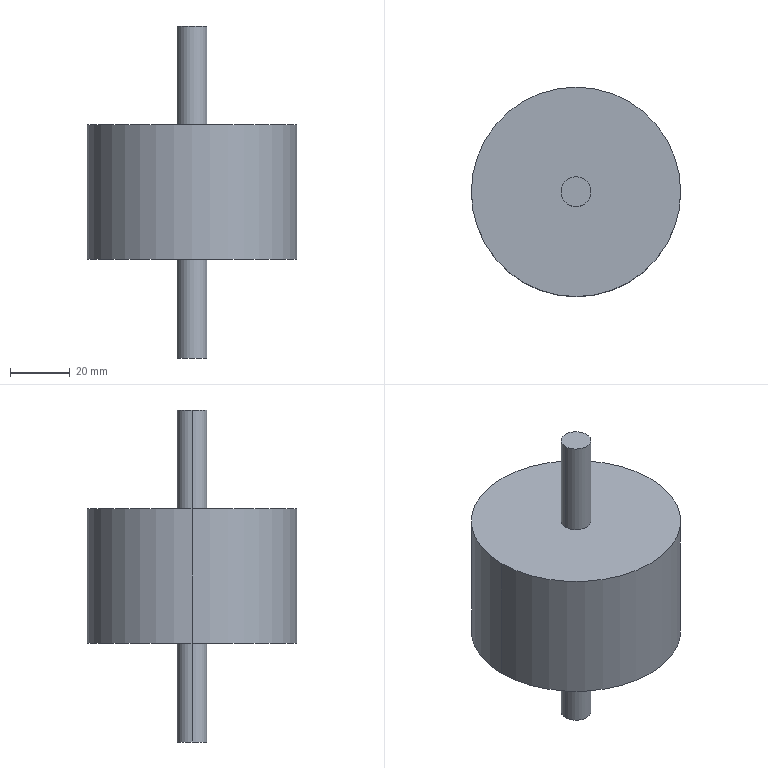Part | 1 solid | 10 faces | box 70 x 70 x 111 mm | volume 178364 mm3 | cylinder 6 | plane 4 | commonest cylinder face diameters 10 x4 70 x2
STEP:
#1=CARTESIAN_POINT('',(-5.,0.,-33.));
#2=VERTEX_POINT('',#1);
#3=CARTESIAN_POINT('',(5.,0.,-33.));
#4=VERTEX_POINT('',#3);
#5=CARTESIAN_POINT('',(0.,0.,-33.));
#6=DIRECTION('',(0.,0.,-1.));
#7=DIRECTION('',(-1.,0.,0.));
#8=AXIS2_PLACEMENT_3D('',#5,#6,#7);
#9=CIRCLE('',#8,5.);
#10=EDGE_CURVE('',#2,#4,#9,.T.);
#11=ORIENTED_EDGE('',*,*,#10,.F.);
#12=CARTESIAN_POINT('',(-5.,0.,0.));
#13=VERTEX_POINT('',#12);
#14=CARTESIAN_POINT('',(-5.,0.,-33.));
#15=DIRECTION('',(0.,0.,1.));
#16=VECTOR('',#15,1000.);
#17=LINE('',#14,#16);
#18=EDGE_CURVE('',#2,#13,#17,.T.);
#19=ORIENTED_EDGE('',*,*,#18,.T.);
#20=CARTESIAN_POINT('',(5.,0.,0.));
#21=VERTEX_POINT('',#20);
#22=CARTESIAN_POINT('',(0.,0.,0.));
#23=DIRECTION('',(0.,0.,-1.));
#24=DIRECTION('',(1.,0.,0.));
#25=AXIS2_PLACEMENT_3D('',#22,#23,#24);
#26=CIRCLE('',#25,5.);
#27=EDGE_CURVE('',#13,#21,#26,.T.);
#28=ORIENTED_EDGE('',*,*,#27,.T.);
#29=CARTESIAN_POINT('',(5.,0.,-33.));
#30=DIRECTION('',(0.,0.,1.));
#31=VECTOR('',#30,1000.);
#32=LINE('',#29,#31);
#33=EDGE_CURVE('',#4,#21,#32,.T.);
#34=ORIENTED_EDGE('',*,*,#33,.F.);
#35=EDGE_LOOP('',(#11,#19,#28,#34));
#36=FACE_OUTER_BOUND('',#35,.T.);
#37=CARTESIAN_POINT('',(0.,0.,-33.));
#38=DIRECTION('',(0.,0.,1.));
#39=DIRECTION('',(1.,0.,0.));
#40=AXIS2_PLACEMENT_3D('',#37,#38,#39);
#41=CYLINDRICAL_SURFACE('',#40,5.);
#42=ADVANCED_FACE('',(#36),#41,.T.);
#43=CARTESIAN_POINT('',(5.,0.,78.));
#44=VERTEX_POINT('',#43);
#45=CARTESIAN_POINT('',(-5.,0.,78.));
#46=VERTEX_POINT('',#45);
#47=CARTESIAN_POINT('',(0.,0.,78.));
#48=DIRECTION('',(0.,0.,1.));
#49=DIRECTION('',(1.,0.,0.));
#50=AXIS2_PLACEMENT_3D('',#47,#48,#49);
#51=CIRCLE('',#50,5.);
#52=EDGE_CURVE('',#44,#46,#51,.T.);
#53=ORIENTED_EDGE('',*,*,#52,.F.);
#54=CARTESIAN_POINT('',(5.,0.,45.));
#55=VERTEX_POINT('',#54);
#56=CARTESIAN_POINT('',(5.,0.,78.));
#57=DIRECTION('',(0.,0.,-1.));
#58=VECTOR('',#57,1000.);
#59=LINE('',#56,#58);
#60=EDGE_CURVE('',#44,#55,#59,.T.);
#61=ORIENTED_EDGE('',*,*,#60,.T.);
#62=CARTESIAN_POINT('',(-5.,0.,45.));
#63=VERTEX_POINT('',#62);
#64=CARTESIAN_POINT('',(0.,0.,45.));
#65=DIRECTION('',(0.,0.,1.));
#66=DIRECTION('',(1.,0.,0.));
#67=AXIS2_PLACEMENT_3D('',#64,#65,#66);
#68=CIRCLE('',#67,5.);
#69=EDGE_CURVE('',#55,#63,#68,.T.);
#70=ORIENTED_EDGE('',*,*,#69,.T.);
#71=CARTESIAN_POINT('',(-5.,0.,78.));
#72=DIRECTION('',(0.,0.,-1.));
#73=VECTOR('',#72,1000.);
#74=LINE('',#71,#73);
#75=EDGE_CURVE('',#46,#63,#74,.T.);
#76=ORIENTED_EDGE('',*,*,#75,.F.);
#77=EDGE_LOOP('',(#53,#61,#70,#76));
#78=FACE_OUTER_BOUND('',#77,.T.);
#79=CARTESIAN_POINT('',(0.,0.,78.));
#80=DIRECTION('',(0.,0.,-1.));
#81=DIRECTION('',(-1.,0.,0.));
#82=AXIS2_PLACEMENT_3D('',#79,#80,#81);
#83=CYLINDRICAL_SURFACE('',#82,5.);
#84=ADVANCED_FACE('',(#78),#83,.T.);
#85=CARTESIAN_POINT('',(35.,0.,45.));
#86=VERTEX_POINT('',#85);
#87=CARTESIAN_POINT('',(-35.,0.,45.));
#88=VERTEX_POINT('',#87);
#89=CARTESIAN_POINT('',(0.,0.,45.));
#90=DIRECTION('',(0.,0.,1.));
#91=DIRECTION('',(1.,0.,0.));
#92=AXIS2_PLACEMENT_3D('',#89,#90,#91);
#93=CIRCLE('',#92,35.);
#94=EDGE_CURVE('',#86,#88,#93,.T.);
#95=ORIENTED_EDGE('',*,*,#94,.F.);
#96=CARTESIAN_POINT('',(35.,0.,0.));
#97=VERTEX_POINT('',#96);
#98=CARTESIAN_POINT('',(35.,0.,45.));
#99=DIRECTION('',(0.,0.,-1.));
#100=VECTOR('',#99,1000.);
#101=LINE('',#98,#100);
#102=EDGE_CURVE('',#86,#97,#101,.T.);
#103=ORIENTED_EDGE('',*,*,#102,.T.);
#104=CARTESIAN_POINT('',(-35.,0.,0.));
#105=VERTEX_POINT('',#104);
#106=CARTESIAN_POINT('',(0.,0.,0.));
#107=DIRECTION('',(0.,0.,1.));
#108=DIRECTION('',(1.,0.,0.));
#109=AXIS2_PLACEMENT_3D('',#106,#107,#108);
#110=CIRCLE('',#109,35.);
#111=EDGE_CURVE('',#97,#105,#110,.T.);
#112=ORIENTED_EDGE('',*,*,#111,.T.);
#113=CARTESIAN_POINT('',(-35.,0.,45.));
#114=DIRECTION('',(0.,0.,-1.));
#115=VECTOR('',#114,1000.);
#116=LINE('',#113,#115);
#117=EDGE_CURVE('',#88,#105,#116,.T.);
#118=ORIENTED_EDGE('',*,*,#117,.F.);
#119=EDGE_LOOP('',(#95,#103,#112,#118));
#120=FACE_OUTER_BOUND('',#119,.T.);
#121=CARTESIAN_POINT('',(0.,0.,45.));
#122=DIRECTION('',(0.,0.,-1.));
#123=DIRECTION('',(-1.,0.,0.));
#124=AXIS2_PLACEMENT_3D('',#121,#122,#123);
#125=CYLINDRICAL_SURFACE('',#124,35.);
#126=ADVANCED_FACE('',(#120),#125,.T.);
#127=ORIENTED_EDGE('',*,*,#102,.F.);
#128=CARTESIAN_POINT('',(0.,0.,45.));
#129=DIRECTION('',(0.,0.,1.));
#130=DIRECTION('',(1.,0.,0.));
#131=AXIS2_PLACEMENT_3D('',#128,#129,#130);
#132=CIRCLE('',#131,35.);
#133=EDGE_CURVE('',#88,#86,#132,.T.);
#134=ORIENTED_EDGE('',*,*,#133,.F.);
#135=ORIENTED_EDGE('',*,*,#117,.T.);
#136=CARTESIAN_POINT('',(0.,0.,0.));
#137=DIRECTION('',(0.,0.,1.));
#138=DIRECTION('',(1.,0.,0.));
#139=AXIS2_PLACEMENT_3D('',#136,#137,#138);
#140=CIRCLE('',#139,35.);
#141=EDGE_CURVE('',#105,#97,#140,.T.);
#142=ORIENTED_EDGE('',*,*,#141,.T.);
#143=EDGE_LOOP('',(#127,#134,#135,#142));
#144=FACE_OUTER_BOUND('',#143,.T.);
#145=CARTESIAN_POINT('',(0.,0.,45.));
#146=DIRECTION('',(0.,0.,-1.));
#147=DIRECTION('',(-1.,0.,0.));
#148=AXIS2_PLACEMENT_3D('',#145,#146,#147);
#149=CYLINDRICAL_SURFACE('',#148,35.);
#150=ADVANCED_FACE('',(#144),#149,.T.);
#151=CARTESIAN_POINT('',(0.,0.,45.));
#152=DIRECTION('',(0.,0.,1.));
#153=DIRECTION('',(1.,0.,0.));
#154=AXIS2_PLACEMENT_3D('',#151,#152,#153);
#155=CIRCLE('',#154,5.);
#156=EDGE_CURVE('',#63,#55,#155,.T.);
#157=ORIENTED_EDGE('',*,*,#156,.F.);
#158=ORIENTED_EDGE('',*,*,#69,.F.);
#159=EDGE_LOOP('',(#157,#158));
#160=FACE_BOUND('',#159,.T.);
#161=ORIENTED_EDGE('',*,*,#133,.T.);
#162=ORIENTED_EDGE('',*,*,#94,.T.);
#163=EDGE_LOOP('',(#161,#162));
#164=FACE_OUTER_BOUND('',#163,.T.);
#165=CARTESIAN_POINT('',(0.,0.,45.));
#166=DIRECTION('',(0.,0.,1.));
#167=DIRECTION('',(1.,0.,0.));
#168=AXIS2_PLACEMENT_3D('',#165,#166,#167);
#169=PLANE('',#168);
#170=ADVANCED_FACE('',(#160,#164),#169,.T.);
#171=CARTESIAN_POINT('',(0.,0.,0.));
#172=DIRECTION('',(0.,0.,-1.));
#173=DIRECTION('',(1.,0.,0.));
#174=AXIS2_PLACEMENT_3D('',#171,#172,#173);
#175=CIRCLE('',#174,5.);
#176=EDGE_CURVE('',#21,#13,#175,.T.);
#177=ORIENTED_EDGE('',*,*,#176,.F.);
#178=ORIENTED_EDGE('',*,*,#27,.F.);
#179=EDGE_LOOP('',(#177,#178));
#180=FACE_BOUND('',#179,.T.);
#181=ORIENTED_EDGE('',*,*,#141,.F.);
#182=ORIENTED_EDGE('',*,*,#111,.F.);
#183=EDGE_LOOP('',(#181,#182));
#184=FACE_OUTER_BOUND('',#183,.T.);
#185=CARTESIAN_POINT('',(0.,0.,0.));
#186=DIRECTION('',(0.,0.,1.));
#187=DIRECTION('',(1.,0.,0.));
#188=AXIS2_PLACEMENT_3D('',#185,#186,#187);
#189=PLANE('',#188);
#190=ADVANCED_FACE('',(#180,#184),#189,.F.);
#191=ORIENTED_EDGE('',*,*,#60,.F.);
#192=CARTESIAN_POINT('',(0.,0.,78.));
#193=DIRECTION('',(0.,0.,1.));
#194=DIRECTION('',(1.,0.,0.));
#195=AXIS2_PLACEMENT_3D('',#192,#193,#194);
#196=CIRCLE('',#195,5.);
#197=EDGE_CURVE('',#46,#44,#196,.T.);
#198=ORIENTED_EDGE('',*,*,#197,.F.);
#199=ORIENTED_EDGE('',*,*,#75,.T.);
#200=ORIENTED_EDGE('',*,*,#156,.T.);
#201=EDGE_LOOP('',(#191,#198,#199,#200));
#202=FACE_OUTER_BOUND('',#201,.T.);
#203=CARTESIAN_POINT('',(0.,0.,78.));
#204=DIRECTION('',(0.,0.,-1.));
#205=DIRECTION('',(-1.,0.,0.));
#206=AXIS2_PLACEMENT_3D('',#203,#204,#205);
#207=CYLINDRICAL_SURFACE('',#206,5.);
#208=ADVANCED_FACE('',(#202),#207,.T.);
#209=ORIENTED_EDGE('',*,*,#197,.T.);
#210=ORIENTED_EDGE('',*,*,#52,.T.);
#211=EDGE_LOOP('',(#209,#210));
#212=FACE_OUTER_BOUND('',#211,.T.);
#213=CARTESIAN_POINT('',(0.,0.,78.));
#214=DIRECTION('',(0.,0.,1.));
#215=DIRECTION('',(1.,0.,0.));
#216=AXIS2_PLACEMENT_3D('',#213,#214,#215);
#217=PLANE('',#216);
#218=ADVANCED_FACE('',(#212),#217,.T.);
#219=ORIENTED_EDGE('',*,*,#18,.F.);
#220=CARTESIAN_POINT('',(0.,0.,-33.));
#221=DIRECTION('',(0.,0.,-1.));
#222=DIRECTION('',(-1.,0.,0.));
#223=AXIS2_PLACEMENT_3D('',#220,#221,#222);
#224=CIRCLE('',#223,5.);
#225=EDGE_CURVE('',#4,#2,#224,.T.);
#226=ORIENTED_EDGE('',*,*,#225,.F.);
#227=ORIENTED_EDGE('',*,*,#33,.T.);
#228=ORIENTED_EDGE('',*,*,#176,.T.);
#229=EDGE_LOOP('',(#219,#226,#227,#228));
#230=FACE_OUTER_BOUND('',#229,.T.);
#231=CARTESIAN_POINT('',(0.,0.,-33.));
#232=DIRECTION('',(0.,0.,1.));
#233=DIRECTION('',(1.,0.,0.));
#234=AXIS2_PLACEMENT_3D('',#231,#232,#233);
#235=CYLINDRICAL_SURFACE('',#234,5.);
#236=ADVANCED_FACE('',(#230),#235,.T.);
#237=ORIENTED_EDGE('',*,*,#225,.T.);
#238=ORIENTED_EDGE('',*,*,#10,.T.);
#239=EDGE_LOOP('',(#237,#238));
#240=FACE_OUTER_BOUND('',#239,.T.);
#241=CARTESIAN_POINT('',(0.,0.,-33.));
#242=DIRECTION('',(0.,0.,-1.));
#243=DIRECTION('',(-1.,0.,0.));
#244=AXIS2_PLACEMENT_3D('',#241,#242,#243);
#245=PLANE('',#244);
#246=ADVANCED_FACE('',(#240),#245,.T.);
#247=CLOSED_SHELL('',(#42,#84,#126,#150,#170,#190,#208,#218,#236,#246));
#248=MANIFOLD_SOLID_BREP('',#247);
#249=CARTESIAN_POINT('',(0.,0.,0.));
#250=DIRECTION('',(0.,0.,1.));
#251=DIRECTION('',(1.,0.,0.));
#252=AXIS2_PLACEMENT_3D('',#249,#250,#251);
#253=(LENGTH_UNIT()NAMED_UNIT(*)SI_UNIT(.MILLI.,.METRE.));
#254=UNCERTAINTY_MEASURE_WITH_UNIT(LENGTH_MEASURE(0.00001),#253,'','');
#255=(NAMED_UNIT(*)PLANE_ANGLE_UNIT()SI_UNIT($,.RADIAN.));
#256=(NAMED_UNIT(*)SI_UNIT($,.STERADIAN.)SOLID_ANGLE_UNIT());
#257=(GEOMETRIC_REPRESENTATION_CONTEXT(3)GLOBAL_UNCERTAINTY_ASSIGNED_CONTEXT((#254))GLOBAL_UNIT_ASSIGNED_CONTEXT((#253,#255,#256))REPRESENTATION_CONTEXT('',''));
#258=ADVANCED_BREP_SHAPE_REPRESENTATION('',(#248,#252),#257);